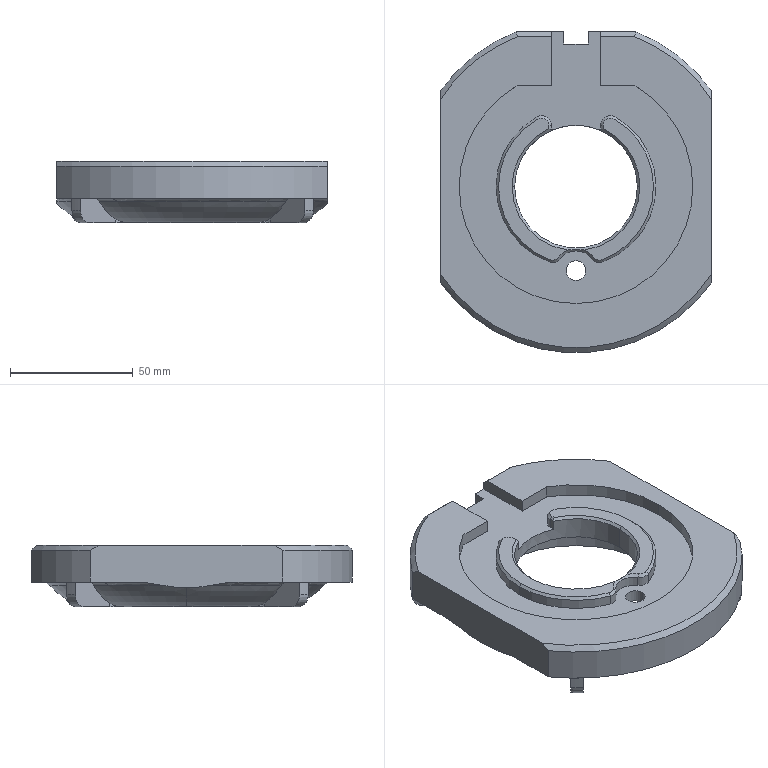Part | SolidWorks | features ICE 8, Chamfer 2, Fillet 2, Extrusion 1, HoleWzd 1, Revolution 1 | 1 solid | 110 faces | box 110 x 130.5 x 25 mm | volume 159387 mm3 | cylinder 42 | plane 38 | cone 18 | torus 12 | commonest cylinder face diameters 8 x16 6.8 x4 84.445 x4 134 x4 65 x3 95 x3